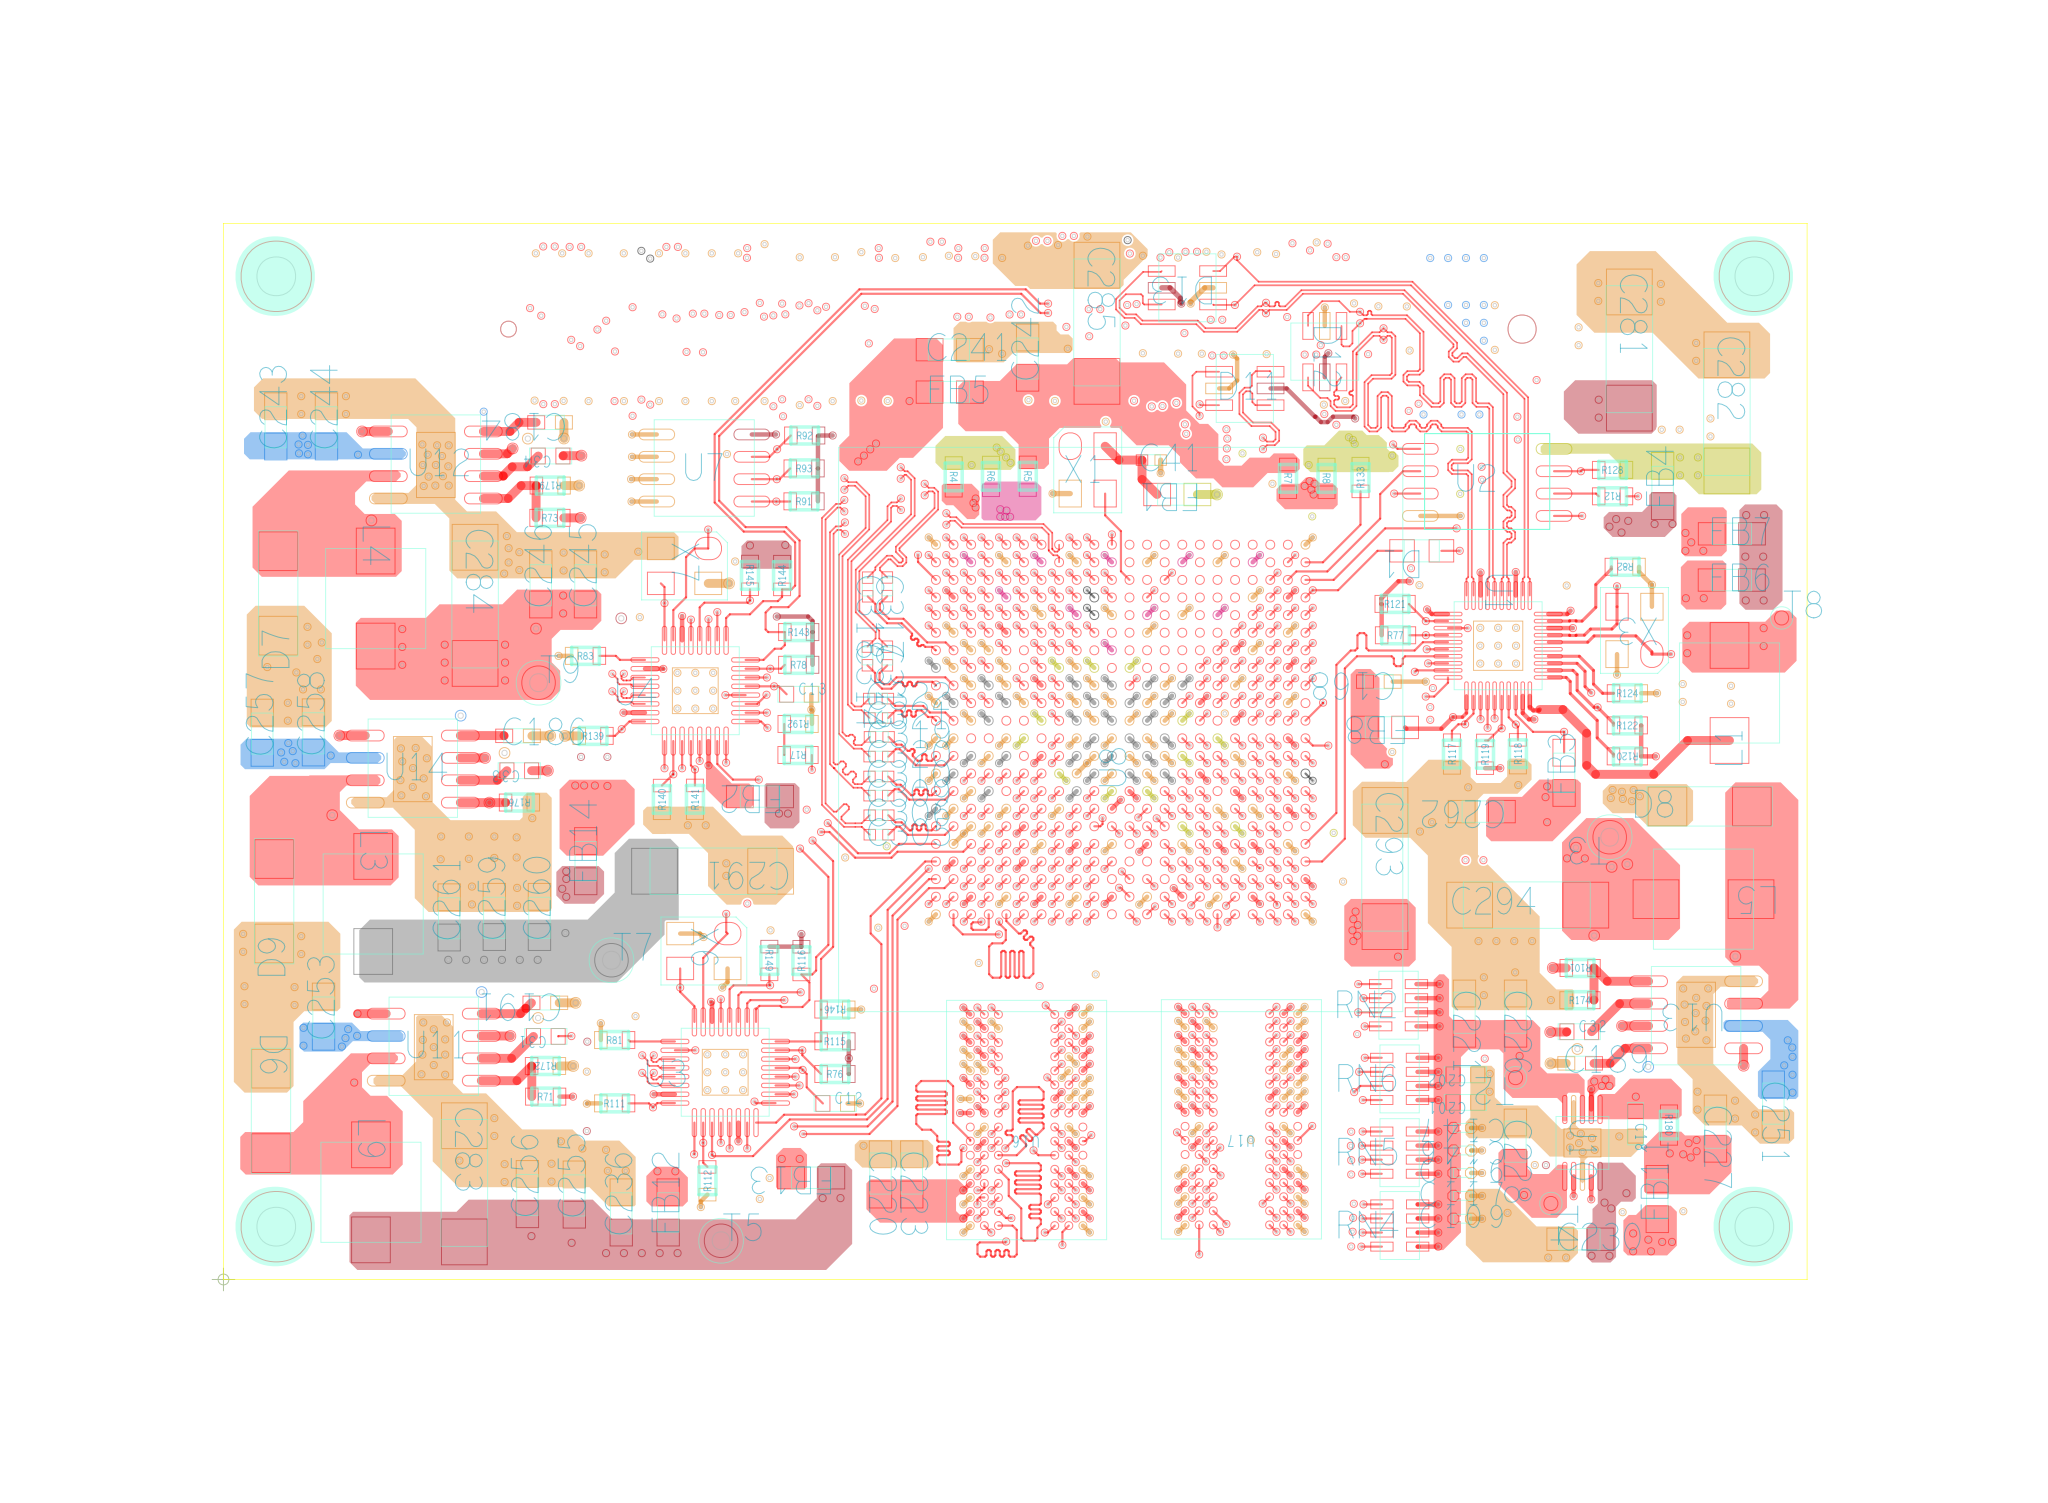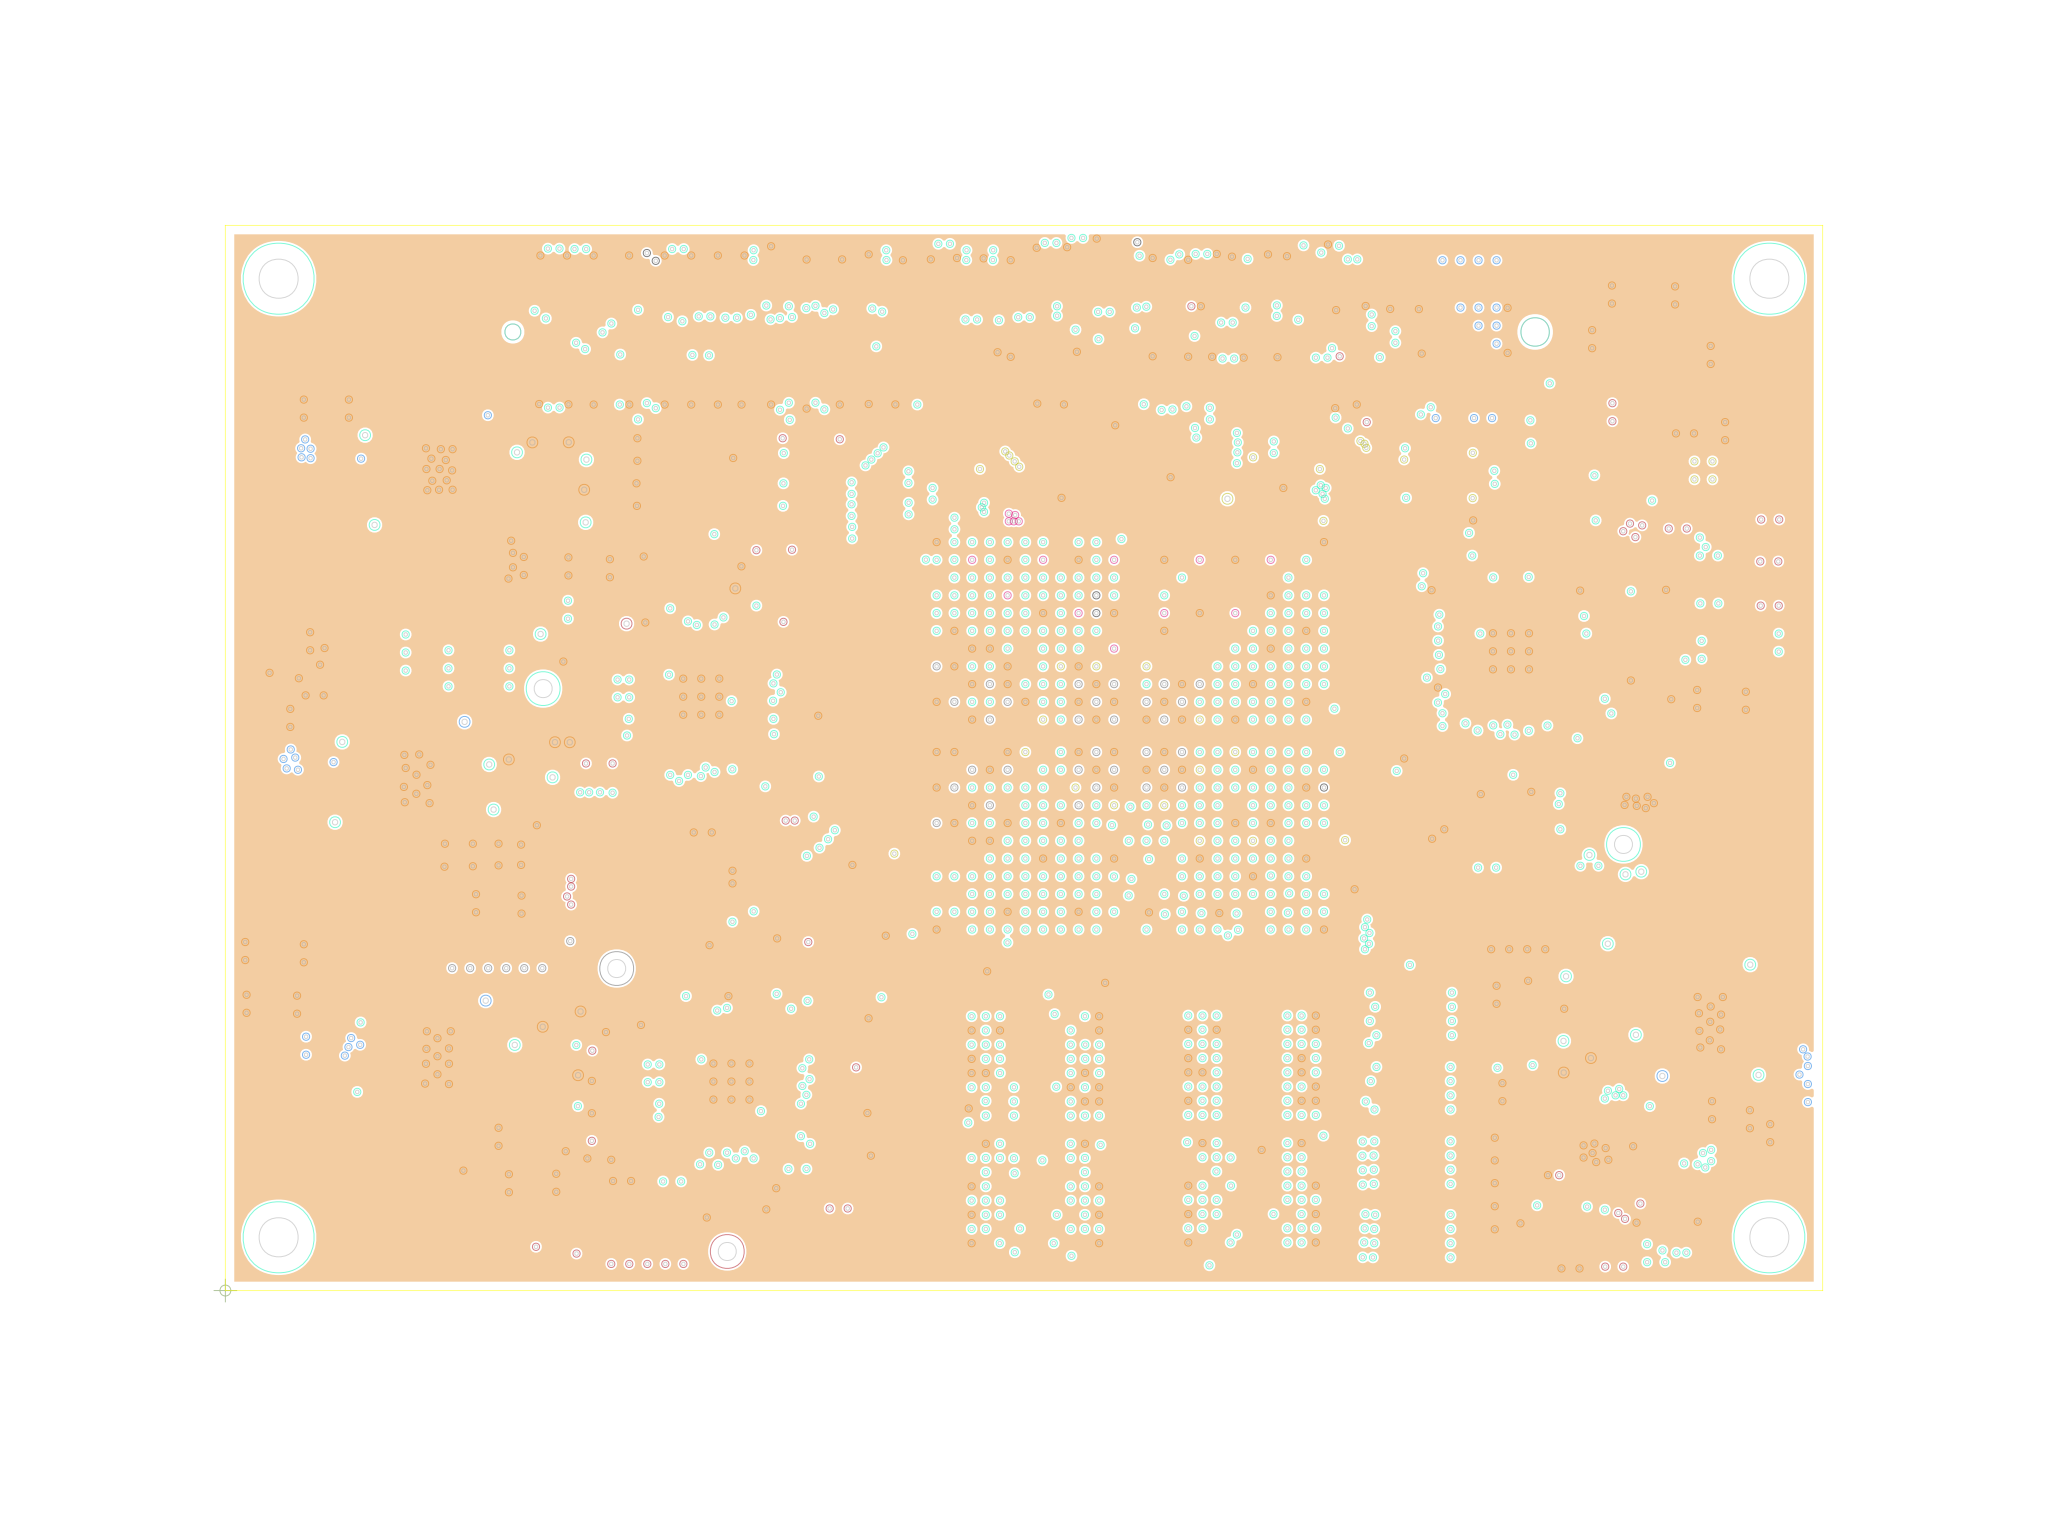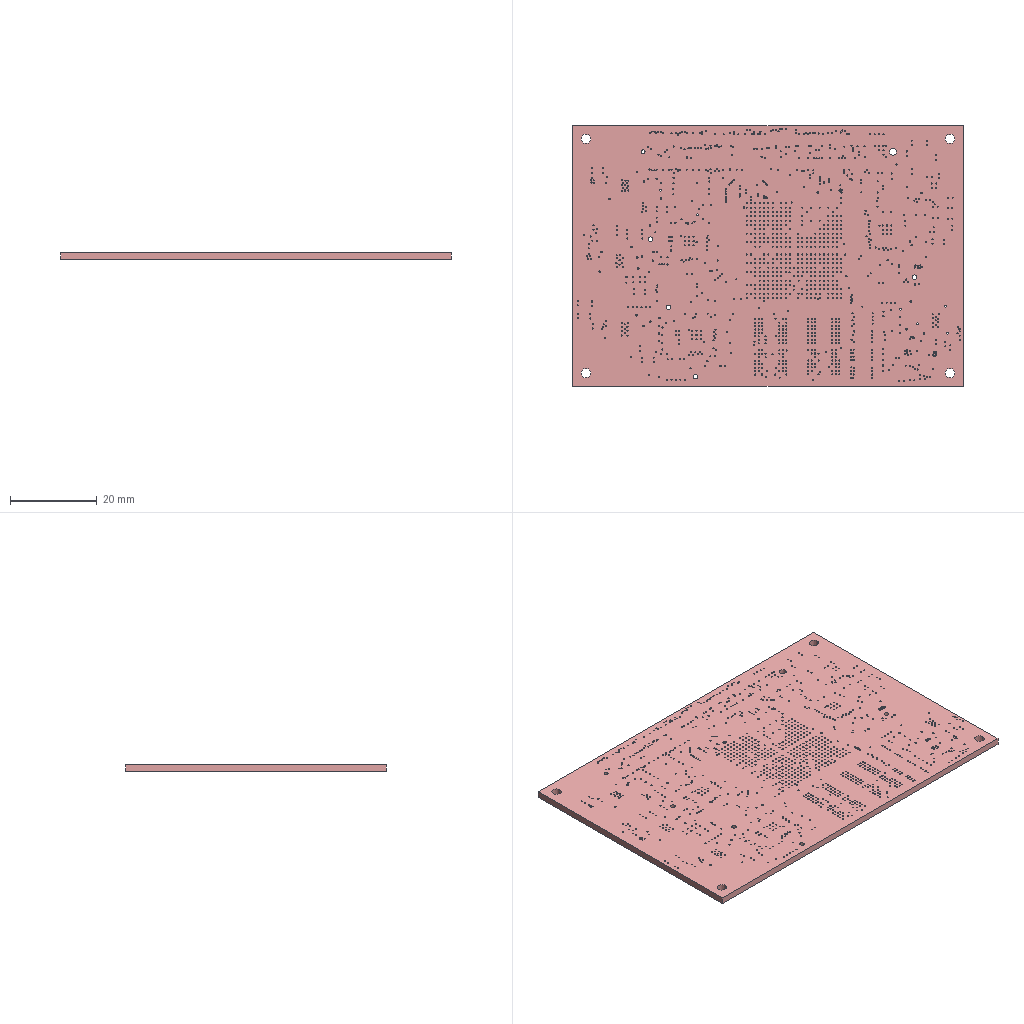Circuit board layout | Cadence Allegro | box 90 x 60 x 1.6 mm
Layer stack:
# Cadence Allegro layer stack of  (unit mm; from the constraint file cross-section; dielectric type: 0 not recorded (Allegro does not mark core vs prepreg), 3 surface material)
index,name,kind,layer,copper_thickness_mm,dielectric_type,dielectric_thickness_mm,dielectric_material,dielectric_constant
0,Top Surface,other,,,,,,
1,TOP,copper,TOP,0.0305,,,,
2,Dielectric1,dielectric,,,0,0.2032,FR-4,4.5
3,GND2,copper,GND2,0.0305,,,,
4,Dielectric2,dielectric,,,0,0.2032,FR-4,4.5
5,SIG3,copper,SIG3,0.0305,,,,
6,Dielectric3,dielectric,,,0,0.2032,FR-4,4.5
7,POWER4,copper,POWER4,0.0305,,,,
8,Dielectric4,dielectric,,,0,0.2032,FR-4,4.5
9,GND5,copper,GND5,0.0305,,,,
10,Dielectric5,dielectric,,,0,0.2032,FR-4,4.5
11,SIG6,copper,SIG6,0.0305,,,,
12,Dielectric6,dielectric,,,0,0.2032,FR-4,4.5
13,POWER7,copper,POWER7,0.0305,,,,
14,Dielectric7,dielectric,,,0,0.2032,FR-4,4.5
15,BOTTOM,copper,BOTTOM,0.0305,,,,
16,Bottom Surface,other,,,,,,
# drill layer pairs: low layer,high layer
drill_pair,TOP,BOTTOM
Part placement:
REFDES,COMP_VALUE,SYM_NAME,SYM_X,SYM_Y,SYM_ROTATE,SYM_MIRROR
C1,10pF,C_0603,1081.558,1609.443,90.000,YES
C2,10pF,C_0603,977.518,1588.167,270.000,YES
C3,10pF,C_0603,1124.854,748.020,90.000,YES
C4,10pF,C_0603,1020.815,726.744,270.000,YES
C6,12pF,C_0603,3147.244,1505.118,180.000,YES
C7,12pF,C_0603,3166.142,1399.606,0.000,YES
C11,100pF,C_0603,2624.185,1510.646,0.000,YES
C12,100pF,C_0603,1368.768,393.717,0.000,NO
C13,100pF,C_0603,1287.652,1309.064,0.000,NO
C14,100pF,C_0603,1655.118,735.654,270.000,YES
C15,100pF,C_0603,2470.000,819.000,90.000,YES
C18,1nF,C_0603,3159.421,348.437,270.000,NO
C21,10nF,C_0603,2905.000,123.999,270.000,YES
C22,10nF,C_0603,364.173,468.110,90.000,YES
C23,10nF,C_0603,3382.724,660.488,270.000,YES
C24,10nF,C_0603,304.504,1066.276,90.000,YES
C25,10nF,C_0603,368.898,1747.472,90.000,YES
C31,22nF,C_0603,721.260,543.701,180.000,NO
C32,22nF,C_0603,3033.465,554.331,0.000,NO
C33,22nF,C_0603,661.811,1138.189,180.000,NO
C34,22nF,C_0603,731.890,1842.126,180.000,NO
C41,100nF_0402,C_0402_104,2076.000,1833.000,0.000,NO
C42,100nF_0402,C_0402_104,3230.000,1849.000,90.000,YES
C44,100nF_0402,C_0402_104,1950.000,1231.000,0.000,YES
C45,100nF_0402,C_0402_104,1866.000,1232.000,0.000,YES
C46,100nF_0402,C_0402_104,1756.000,1273.000,180.000,YES
C47,100nF_0402,C_0402_104,1606.000,1424.000,180.000,YES
C48,100nF_0402,C_0402_104,1600.000,1148.000,0.000,YES
C49,100nF_0402,C_0402_104,1597.000,1335.000,0.000,YES
C50,100nF_0402,C_0402_104,1720.000,1075.000,180.000,YES
C51,100nF_0402,C_0402_104,1892.000,1365.000,270.000,YES
C52,100nF_0402,C_0402_104,985.000,1030.000,180.000,YES
C53,100nF_0402,C_0402_104,2031.000,1231.000,0.000,YES
C54,100nF_0402,C_0402_104,1715.000,1231.000,180.000,YES
C55,100nF_0402,C_0402_104,1599.000,1067.000,180.000,YES
C56,100nF_0402,C_0402_104,1676.000,1186.000,180.000,YES
C57,100nF_0402,C_0402_104,2112.000,1231.000,180.000,YES
C58,100nF_0402,C_0402_104,2010.000,1174.000,90.000,YES
C59,100nF_0402,C_0402_104,1715.000,1345.000,180.000,YES
C60,100nF_0402,C_0402_104,2100.000,1305.000,0.000,YES
C61,100nF_0402,C_0402_104,2120.000,1135.000,270.000,YES
C62,100nF_0402,C_0402_104,2080.000,1135.000,90.000,YES
C63,100nF_0402,C_0402_104,1930.000,1135.000,270.000,YES
C64,100nF_0402,C_0402_104,2100.000,1195.000,0.000,YES
C65,100nF_0402,C_0402_104,1935.000,1325.000,270.000,YES
C66,100nF_0402,C_0402_104,1740.000,1170.000,270.000,YES
C67,100nF_0402,C_0402_104,1970.000,1135.000,90.000,YES
C68,100nF_0402,C_0402_104,1890.000,1170.000,270.000,YES
C69,100nF_0402,C_0402_104,2140.000,1345.000,0.000,YES
C70,100nF_0402,C_0402_104,2045.000,1135.000,270.000,YES
C71,100nF_0402,C_0402_104,1950.000,1195.000,180.000,YES
C72,100nF_0402,C_0402_104,1625.000,1230.000,0.000,YES
C73,100nF_0402,C_0402_104,2010.000,1292.000,90.000,YES
C74,100nF_0402,C_0402_104,2062.000,928.000,0.000,YES
C75,100nF_0402,C_0402_104,1580.000,215.000,270.000,YES
C76,100nF_0402,C_0402_104,1951.000,998.000,180.000,YES
C77,100nF_0402,C_0402_104,2400.000,690.000,180.000,YES
C78,100nF_0402,C_0402_104,1580.000,120.000,90.000,YES
C79,100nF_0402,C_0402_104,2055.000,115.000,90.000,YES
C80,100nF_0402,C_0402_104,2500.000,481.000,90.000,YES
C81,100nF_0402,C_0402_104,2283.000,820.000,90.000,YES
C82,100nF_0402,C_0402_104,2495.000,105.000,90.000,YES
C83,100nF_0402,C_0402_104,2500.000,565.000,270.000,YES
C84,100nF_0402,C_0402_104,2260.000,1265.000,0.000,YES
C85,100nF_0402,C_0402_104,2300.000,1425.000,180.000,YES
C86,100nF_0402,C_0402_104,2465.000,1685.000,90.000,YES
C87,100nF_0402,C_0402_104,2460.000,890.000,180.000,YES
C88,100nF_0402,C_0402_104,2400.000,1565.000,270.000,YES
C89,100nF_0402,C_0402_104,2510.000,1430.000,270.000,YES
C90,100nF_0402,C_0402_104,2240.000,1060.000,90.000,YES
C91,100nF_0402,C_0402_104,2300.000,940.000,45.000,YES
C92,100nF_0402,C_0402_104,2470.000,1430.000,270.000,YES
C93,100nF_0402,C_0402_104,2465.000,1585.000,270.000,YES
C94,100nF_0402,C_0402_104,2395.000,980.000,90.000,YES
C95,100nF_0402,C_0402_104,2035.000,1622.000,180.000,YES
C96,100nF_0402,C_0402_104,2013.000,1527.000,90.000,YES
C97,100nF_0402,C_0402_104,2203.000,1592.000,180.000,YES
C98,100nF_0402,C_0402_104,2035.000,1655.000,180.000,YES
C99,100nF_0402,C_0402_104,2035.000,1589.000,180.000,YES
C100,100nF_0402,C_0402_104,2214.000,1473.000,0.000,YES
C101,100nF_0402,C_0402_104,1992.000,1464.000,180.000,YES
C102,100nF_0402,C_0402_104,2212.000,1529.000,0.000,YES
C103,100nF_0402,C_0402_104,2131.000,1529.000,180.000,YES
C104,100nF_0402,C_0402_104,2202.000,1649.000,180.000,YES
C105,100nF_0402,C_0402_104,1800.000,1145.000,0.000,YES
C106,100nF_0402,C_0402_BGA,2771.000,494.000,0.000,YES
C107,100nF_0402,C_0402_BGA,2770.933,394.571,180.000,YES
C108,100nF_0402,C_0402_BGA,2770.866,83.071,180.000,YES
C109,100nF_0402,C_0402_BGA,2771.654,135.827,0.000,NO
C110,100nF_0402,C_0402_BGA,2771.260,135.433,180.000,YES
C111,100nF_0402,C_0402_BGA,2771.654,187.402,180.000,YES
C112,100nF_0402,C_0402_BGA,2771.260,238.189,180.000,YES
C113,100nF_0402,C_0402_BGA,2771.654,288.583,180.000,YES
C114,100nF_0402,C_0402_BGA,2770.866,338.976,180.000,YES
C115,100nF_0402,C_0402_BGA,2770.866,443.701,180.000,YES
C116,100nF_0402,C_0402_BGA,2771.654,238.189,0.000,NO
C117,100nF_0402,C_0402_BGA,2771.654,187.008,0.000,NO
C121,100nF_0402,C_0402_BGA,1822.033,216.529,270.000,YES
C122,100nF_0402,C_0402_BGA,2685.000,760.000,270.000,YES
C123,100nF_0402,C_0402_BGA,1622.001,216.000,90.000,YES
C124,100nF_0402,C_0402_BGA,1973.001,585.000,90.000,YES
C125,100nF_0402,C_0402_BGA,1973.001,496.000,90.000,YES
C126,100nF_0402,C_0402_BGA,1973.001,408.000,90.000,YES
C127,100nF_0402,C_0402_BGA,2096.000,526.000,270.000,YES
C128,100nF_0402,C_0402_BGA,2096.000,615.000,270.000,YES
C129,100nF_0402,C_0402_BGA,2100.000,215.000,90.000,YES
C130,100nF_0402,C_0402_BGA,2099.000,116.000,270.000,YES
C131,100nF_0402,C_0402_BGA,1618.000,480.000,90.000,YES
C132,100nF_0402,C_0402_BGA,2022.000,586.000,90.000,YES
C133,100nF_0402,C_0402_BGA,1834.000,404.000,90.000,YES
C134,100nF_0402,C_0402_BGA,1618.000,568.000,90.000,YES
C135,100nF_0402,C_0402_BGA,2456.000,474.000,270.000,YES
C136,100nF_0402,C_0402_BGA,2455.000,565.000,90.000,YES
C137,100nF_0402,C_0402_BGA,2452.000,107.000,270.000,YES
C138,100nF_0402,C_0402_BGA,2400.000,646.000,0.000,YES
C139,100nF_0402,C_0402_BGA,1622.000,119.000,270.000,YES
C140,100nF_0402,C_0402_BGA,1978.000,110.000,270.000,YES
C141,100nF_0402,C_0402_BGA,3241.000,133.000,90.000,YES
C142,100nF_0402,C_0402_BGA,3237.008,337.402,90.000,YES
C143,100nF_0402,C_0402_BGA,2900.000,600.000,90.000,YES
C144,100nF_0402,C_0402_BGA,2910.000,235.000,90.000,YES
C145,100nF_0402,C_0402_BGA,3085.000,120.000,90.000,YES
C146,100nF_0402,C_0402_BGA,2772.047,288.583,180.000,NO
C147,100nF_0402,C_0402_BGA,2771.654,338.976,180.000,NO
C148,100nF_0402,C_0402_BGA,2298.815,266.665,90.000,YES
C149,100nF_0402,C_0402_BGA,1618.164,391.728,90.000,YES
C150,100nF_0402,C_0402_BGA,2094.484,393.169,90.000,YES
C151,100nF_0402,C_0402_104,1807.000,1208.000,270.000,YES
C153,100nF_0402,C_0402_104,1795.000,1325.000,45.000,YES
C154,100nF_0402,C_0402_104,1720.000,1445.000,45.000,YES
C155,100nF_0402,C_0402_104,1559.000,1583.000,0.000,YES
C156,100nF_0402,C_0402_104,1774.000,1405.000,90.000,YES
C161,100nF_0603,C_0603_104,2964.244,1383.173,270.000,YES
C162,100nF_0603,C_0603_104,2964.890,1521.362,90.000,YES
C163,100nF_0603,C_0603_104,2890.622,1516.228,270.000,YES
C164,100nF_0603,C_0603_104,2738.654,1457.362,270.000,YES
C165,100nF_0603,C_0603_104,2811.488,1515.819,270.000,YES
C166,100nF_0603,C_0603_104,3413.850,1360.890,270.000,YES
C167,100nF_0603,C_0603_104,2503.000,1159.000,0.000,YES
C168,100nF_0603,C_0603_104,2585.039,1337.402,180.000,NO
C169,100nF_0603,C_0603_104,2675.000,1150.000,180.000,YES
C170,100nF_0603,C_0603_104,2898.102,1171.488,270.000,YES
C171,100nF_0603,C_0603_104,2999.677,1146.480,270.000,YES
C172,100nF_0603,C_0603_104,1038.000,387.000,180.000,YES
C173,100nF_0603,C_0603_104,1029.520,589.047,0.000,YES
C174,100nF_0603,C_0603_104,1011.346,481.299,90.000,YES
C175,100nF_0603,C_0603_104,1074.000,695.000,270.000,YES
C176,100nF_0603,C_0603_104,1170.000,215.000,270.000,YES
C177,100nF_0603,C_0603_104,942.835,1193.488,90.000,YES
C178,100nF_0603,C_0603_104,1053.536,1205.118,180.000,YES
C179,100nF_0603,C_0603_104,962.583,1442.591,0.000,YES
C180,100nF_0603,C_0603_104,944.410,1334.843,90.000,YES
C181,100nF_0603,C_0603_104,1107.071,1442.055,180.000,YES
C182,100nF_0603,C_0603_104,1177.925,1860.079,90.000,YES
C183,100nF_0603,C_0603_104,233.173,1922.165,270.000,YES
C184,100nF_0603,C_0603_104,730.709,1917.323,180.000,NO
C185,100nF_0603,C_0603_104,204.094,1237.638,270.000,YES
C186,100nF_0603,C_0603_104,659.055,1216.142,0.000,NO
C187,100nF_0603,C_0603_104,606.000,815.000,270.000,YES
C188,100nF_0603,C_0603_104,3468.000,557.000,270.000,YES
C189,100nF_0603,C_0603_104,3035.433,483.465,0.000,NO
C190,100nF_0603,C_0603_104,3035.039,625.984,0.000,YES
C191,100nF_0603,C_0603_104,720.079,618.898,180.000,NO
C192,100nF_0603,C_0603_104,780.000,150.000,90.000,YES
C193,100nF_0603,C_0603_104,226.646,601.772,270.000,YES
C201,1uF,C_0603,2778.740,396.063,180.000,NO
C202,1uF,C_0603,2778.740,457.874,180.000,NO
C203,1uF,C_0603,1784.999,400.000,90.000,YES
C204,1uF,C_0603,1530.000,110.000,270.000,YES
C205,1uF,C_0603,1530.000,225.000,90.000,YES
C206,1uF,C_0603,2050.000,220.001,90.000,YES
C207,1uF,C_0603,2033.090,399.736,90.000,YES
C208,1uF,C_0603,1556.377,399.696,90.000,YES
C220,10uF/25V,C_0805_106,1470.000,235.000,270.000,NO
C221,10uF/25V,C_0805_106,2776.563,594.669,270.000,NO
C222,10uF/25V,C_0805_106,2776.000,625.000,90.000,YES
C223,10uF/25V,C_0805_106,1540.000,235.000,270.000,NO
C224,10uF/25V,C_0805_106,1440.000,205.000,90.000,YES
C225,10uF/25V,C_0805_106,2540.000,710.000,180.000,YES
C226,10uF/25V,C_0805_106,2890.925,594.732,270.000,NO
C227,10uF/25V,C_0805_106,3338.169,337.457,270.000,NO
C228,10uF/25V,C_0805_106,2890.531,306.165,270.000,NO
C229,10uF/25V,C_0805_106,3338.583,337.402,90.000,YES
C230,10uF/25V,C_0805_106,3036.000,90.000,0.000,NO
C231,10uF/25V,C_0805_106,3375.079,1564.559,0.000,YES
C232,10uF/25V,C_0805_106,3373.614,1668.760,0.000,YES
C233,10uF/25V,C_0805_106,3313.406,1357.961,90.000,YES
C234,10uF/25V,C_0805_106,2598.819,1235.039,180.000,YES
C236,10uF/25V,C_0805_106,890.000,150.000,90.000,NO
C237,10uF/25V,C_0805_106,1255.000,150.000,270.000,YES
C238,10uF/25V,C_0805_106,809.823,935.331,270.000,YES
C239,10uF/25V,C_0805_106,1199.913,1081.083,0.000,YES
C240,10uF/25V,C_0805_106,3365.748,1853.543,270.000,YES
C241,10uF/25V,C_0805_106,1625.000,2080.000,0.000,NO
C242,10uF/25V,C_0805_106,1799.213,2062.205,90.000,NO
C243,10uF/25V,C_0805_106,117.031,1908.386,90.000,NO
C244,10uF/25V,C_0805_106,230.417,1908.386,90.000,NO
C245,10uF/25V,C_0805_106,810.000,1555.000,90.000,NO
C246,10uF/25V,C_0805_106,710.000,1555.000,90.000,NO
C247,10uF/25V,C_0805_106,3011.024,851.575,90.000,YES
C248,10uF/25V,C_0805_106,2799.213,847.638,90.000,YES
C249,10uF/25V,C_0805_106,2907.480,846.457,90.000,YES
C250,10uF/25V,C_0805_106,3468.394,390.976,90.000,YES
C251,10uF/25V,C_0805_106,3467.606,391.370,270.000,NO
C252,10uF/25V,C_0805_106,99.087,587.205,270.000,YES
C253,10uF/25V,C_0805_106,223.890,587.992,90.000,NO
C254,10uF/25V,C_0805_106,871.000,152.000,270.000,YES
C255,10uF/25V,C_0805_106,785.000,190.000,90.000,NO
C256,10uF/25V,C_0805_106,680.000,191.000,90.000,NO
C257,10uF/25V,C_0805_106,86.772,1223.071,90.000,NO
C258,10uF/25V,C_0805_106,201.339,1223.858,90.000,NO
C259,10uF/25V,C_0805_106,606.000,811.000,90.000,NO
C260,10uF/25V,C_0805_106,707.000,811.000,90.000,NO
C261,10uF/25V,C_0805_106,505.000,810.000,90.000,NO
C262,10uF/25V,C_0805_106,2815.378,1046.626,180.000,NO
C281,100uF/6.3Vdc,C_7343,3145.563,2079.149,270.000,NO
C282,100uF/6.3Vdc,C_7343,3363.780,1938.583,270.000,NO
C283,100uF/6.3Vdc,C_7343,539.000,213.999,270.000,NO
C284,100uF/6.3Vdc,C_7343,563.000,1507.999,270.000,NO
C285,100uF/6.3Vdc,C_7343,1954.331,2138.976,270.000,NO
C291,330uF/2.5Vdc,C_7343,1094.338,913.202,180.000,NO
C292,330uF/2.5Vdc,C_7343,1092.901,912.989,0.000,YES
C293,330uF/2.5Vdc,C_7343,2598.819,919.290,270.000,NO
C294,330uF/2.5Vdc,C_7343,2918.110,837.402,0.000,NO
C302,10uF/25V,C_0805_106,3143.595,1994.897,270.000,YES
C303,100nF_0402,C_0402_104,1466.550,1081.918,180.000,YES
C304,100nF_0402,C_0402_104,1466.550,1125.225,180.000,YES
C305,100nF_0402,C_0402_104,1466.944,994.910,0.000,NO
C306,100nF_0402,C_0402_104,1466.629,1038.595,0.000,NO
C307,100nF_0402,C_0402_104,1466.550,1169.713,180.000,YES
C308,100nF_0402,C_0402_104,1467.337,1213.808,180.000,YES
C309,100nF_0402,C_0402_104,1466.456,1082.296,0.000,NO
C310,100nF_0402,C_0402_104,1466.267,1125.209,0.000,NO
C311,100nF_0402,C_0402_104,1465.369,1344.910,180.000,YES
C312,100nF_0402,C_0402_104,1466.156,1389.792,180.000,YES
C313,100nF_0402,C_0402_104,1485.298,1394.693,270.000,NO
C314,100nF_0402,C_0402_104,1440.809,1394.882,270.000,NO
C315,100nF_0402,C_0402_104,1466.156,1435.067,180.000,YES
C316,100nF_0402,C_0402_104,1465.369,1479.162,180.000,YES
C317,100nF_0402,C_0402_104,1485.230,1549.503,270.000,NO
C318,100nF_0402,C_0402_104,1441.371,1549.125,270.000,NO
C319,100nF_0402,C_0402_104,1467.338,1213.841,0.000,NO
C320,100nF_0402,C_0402_104,1466.549,1169.680,0.000,NO
C321,100nF_0402,C_0402_104,1466.204,1256.091,0.000,NO
C322,100nF_0402,C_0402_104,1465.621,1299.398,0.000,NO
D1,R_LED_SMT,D_LED0805,2681.001,1630.001,180.000,NO
D6,SS210,DO214,106.299,377.165,270.000,NO
D7,SS210,DO214,122.441,1534.646,90.000,NO
D8,SS210,DO214,3325.197,1058.268,0.000,NO
D9,SS210,DO214,113.386,846.063,90.000,NO
D11,SRV05-4,D_SOT23_6,2285.200,1993.246,0.000,NO
D12,SRV05-4,D_SOT23_6,2464.076,2075.592,270.000,NO
D13,SRV05-4,D_SOT23_6,2156.756,2218.426,180.000,NO
FB1,CBW201209U600T,L_0805,2134.000,1756.000,180.000,NO
FB2,CBW201209U600T,L_0805,1200.394,1080.315,180.000,NO
FB3,CBW201209U600T,L_0805,2999.524,1133.394,90.000,NO
FB4,CBW201209U600T,L_0805,3220.000,1775.000,90.000,NO
FB5,CBW201209U600T,L_0805,1625.000,1985.000,0.000,NO
FB6,CBW201209U600T,L_0805,3374.685,1564.559,0.000,NO
FB7,CBW201209U600T,L_0805,3374.898,1668.055,0.000,NO
FB8,CBW201209U600T,L_0805,2598.732,1234.957,180.000,NO
FB10,CBW201209U600T,L_0805,2604.331,874.409,90.000,YES
FB11,CBW201209U600T,L_0805,3208.000,180.000,90.000,NO
FB12,CBW201209U600T,L_0805,995.000,150.000,90.000,NO
FB13,CBW201209U600T,L_0805,1314.961,227.559,180.000,NO
FB14,CBW201209U600T,L_0805,810.547,935.787,90.000,NO
J10,COM_E connector 220X8 FEMALE,JP_220X8PF,1771.654,2125.984,90.000,YES
L1,2.2uH,L_SDB0530,3369.642,1312.016,90.000,NO
L3,3.3uH,L_SDB0530,335.000,840.000,270.000,NO
L4,3.3uH,L_SDB0530,340.551,1523.228,270.000,NO
L5,3.3uH,L_SDB0530,3311.417,850.787,180.000,NO
L9,4.7uH,L_SDB0530,330.000,195.000,270.000,NO
R1,0,R_0603,1582.677,732.110,90.000,YES
R2,0,R_0603,2184.506,710.691,90.000,YES
R3,0,R_0603,1782.286,713.774,270.000,YES
R4,0,R_0603,1633.858,1795.410,270.000,NO
R5,0,R_0603,1799.606,1796.850,270.000,NO
R6,0,R_0603,1717.154,1796.457,270.000,NO
R7,0,R_0603,2381.890,1792.126,270.000,NO
R8,0,R_0603,2468.000,1792.000,270.000,NO
R9,0,R_0603,2105.000,1400.000,0.000,YES
R10,0,R_0603,2009.000,1383.000,90.000,YES
R11,10,R_0603,3015.000,129.000,270.000,YES
R12,10,R_0603,3108.000,1752.000,180.000,NO
R13,10,R_0603,364.173,587.402,270.000,YES
R14,10,R_0603,3382.724,541.197,90.000,YES
R15,10,R_0603,304.504,1185.567,270.000,YES
R16,10,R_0603,368.898,1866.764,270.000,YES
R17,10,R_0603,1285.505,1173.281,180.000,NO
R21,33.2,R_0603,2632.323,407.066,0.000,YES
R22,33.2,R_0603,2632.039,478.325,0.000,YES
R23,33.2,R_0603,2630.873,548.778,180.000,YES
R26,499,R_0603,659.843,1138.189,180.000,YES
R31,80.6,R_0603,878.000,532.000,0.000,YES
R32,80.6,R_0603,877.000,332.000,0.000,YES
R41,49.9,R_0603,854.000,1448.000,270.000,YES
R42,49.9,R_0603,794.000,1448.000,270.000,YES
R43,49.9,R_0603,859.000,1228.000,90.000,YES
R44,49.9,R_0603,800.000,1228.000,90.000,YES
R51,130,R_0603,876.717,393.248,180.000,YES
R52,130,R_0603,877.220,464.902,180.000,YES
R56,243,R_0603,1986.271,228.346,90.000,YES
R57,243,R_0603,2466.528,233.464,90.000,YES
R58,243,R_0603,1852.217,713.790,270.000,YES
R59,243,R_0603,1921.222,713.397,270.000,YES
R61,1K,R_0603,2955.000,129.000,90.000,YES
R62,1K,R_0603,2688.000,1628.000,180.000,YES
R64,1K,R_0603,2397.000,1715.000,270.000,YES
R65,1K,R_0603,2338.000,1715.000,270.000,YES
R66,1K,R_0603,1425.000,913.000,270.000,YES
R67,1K,R_0603,1484.000,913.000,90.000,YES
R71,1.21K,R_0603,720.866,409.055,0.000,NO
R73,1.24K,R_0603,730.449,1703.736,0.000,NO
R76,1.5K,R_0603,1368.134,459.642,0.000,NO
R77,1.5K,R_0603,2622.354,1441.138,0.000,NO
R78,1.5K,R_0603,1287.019,1374.989,0.000,NO
R81,2.49K,R_0603,875.283,535.626,0.000,NO
R82,2.49K,R_0603,3136.244,1594.295,180.000,NO
R83,2.49K,R_0603,810.000,1395.000,0.000,NO
R91,3.32K,R_0603,1298.969,1740.744,0.000,NO
R92,3.32K,R_0603,1300.433,1887.988,0.000,NO
R93,3.32K,R_0603,1299.142,1814.366,0.000,NO
R94,3.32K,R_0603,3036.220,553.543,0.000,YES
R95,3.32K,R_0603,729.134,1842.913,180.000,YES
R96,3.32K,R_0603,718.504,544.488,180.000,YES
R101,4.02K,R_0603,3035.433,696.850,180.000,NO
R111,4.75K,R_0603,875.300,394.000,0.000,NO
R112,4.75K,R_0603,1082.846,220.748,90.000,NO
R113,4.75K,R_0603,1103.000,210.000,270.000,YES
R115,4.75K,R_0603,1368.165,532.902,0.000,NO
R116,4.75K,R_0603,1293.083,713.331,90.000,NO
R117,4.75K,R_0603,2748.594,1175.425,90.000,NO
R118,4.75K,R_0603,2896.232,1176.102,90.000,NO
R119,4.75K,R_0603,2822.610,1174.811,90.000,NO
R120,4.75K,R_0603,3140.968,1170.180,180.000,NO
R121,4.75K,R_0603,2621.441,1511.248,0.000,NO
R122,4.75K,R_0603,3140.952,1239.506,0.000,NO
R123,4.75K,R_0603,3140.944,1239.424,180.000,YES
R124,4.75K,R_0603,3141.126,1311.500,0.000,NO
R125,4.75K,R_0603,1524.000,732.000,270.000,YES
R126,4.75K,R_0603,2687.555,1857.868,180.000,YES
R127,4.75K,R_0603,2687.161,1757.473,180.000,YES
R128,4.75K,R_0603,3108.000,1811.000,0.000,NO
R132,4.75K,R_0603,2521.000,969.000,270.000,YES
R133,4.75K,R_0603,2544.000,1794.000,90.000,NO
R134,4.75K,R_0603,2448.000,968.000,270.000,YES
R139,4.75K,R_0603,827.000,1216.000,0.000,NO
R140,4.75K,R_0603,980.878,1073.898,90.000,NO
R141,4.75K,R_0603,1054.894,1074.181,90.000,NO
R142,4.75K,R_0603,1177.881,1575.211,90.000,YES
R143,4.75K,R_0603,1287.050,1448.249,0.000,NO
R144,4.75K,R_0603,1249.786,1574.754,90.000,NO
R145,4.75K,R_0603,1178.046,1575.037,270.000,NO
R146,4.75K,R_0603,1368.008,603.854,180.000,NO
R147,4.75K,R_0603,1224.000,720.000,90.000,YES
R148,4.75K,R_0603,3035.827,696.850,180.000,YES
R149,4.75K,R_0603,1221.343,713.614,270.000,NO
R161,5.11K,R_0603,662.205,1066.929,180.000,YES
R171,10K,R_0603,577.559,575.591,90.000,YES
R172,10K,R_0603,720.472,477.559,180.000,NO
R173,10K,R_0603,3187.795,536.220,270.000,YES
R174,10K,R_0603,3035.039,624.803,0.000,NO
R175,10K,R_0603,530.709,1197.638,90.000,YES
R176,10K,R_0603,662.205,1066.929,180.000,NO
R177,10K,R_0603,2989.890,221.768,180.000,YES
R178,10K,R_0603,582.283,1877.953,90.000,YES
R179,10K,R_0603,731.102,1775.984,180.000,NO
R180,10K,R_0603,3234.193,345.425,270.000,NO
R181,10K,R_0603,3228.000,419.000,180.000,YES
R191,20K,R_0603,730.291,1703.878,0.000,YES
R192,20K,R_0603,1285.710,1242.683,180.000,NO
R196,30.1K,R_0603,720.079,409.055,0.000,YES
R199,100K,R_0603,3108.000,221.000,180.000,YES
R200,4.75K,R_0603,3140.968,1311.626,180.000,YES
R201,4.75K,R_0603,1465.000,732.000,90.000,YES
RN1,33,RESNET4,2631.511,283.734,180.000,YES
RN2,33,RESNET4,2629.147,613.530,0.000,NO
RN3,33,RESNET4,2631.511,121.135,180.000,YES
RN4,33,RESNET4,2631.904,120.742,0.000,NO
RN5,33,RESNET4,2631.511,283.734,0.000,NO
RN6,33,RESNET4,2631.511,448.694,0.000,NO
T1,TP_0_8,TP_0_8,1712.000,732.000,0.000,YES
T2,TP_0_8,TP_0_8,2890.945,451.575,180.000,NO
T3,1.5V 3A,TP,3101.575,989.370,180.000,NO
T4,TP_0_8,TP_0_8,2970.000,170.000,270.000,NO
T5,3.3V  2A,TP,1113.386,86.614,0.000,NO
T7,1.2V 1A,TP,868.110,714.173,0.000,NO
T8,TP_0_8,TP_0_8,3486.220,1479.921,0.000,NO
T9,2.5V 1A,TP,705.000,1335.000,0.000,NO
U1,RTL8211FI-CG,U_QFN40_0_4,2851.969,1417.717,270.000,NO
U2,W25Q64FVSSIG,U_SO8W,2827.436,1783.064,0.000,NO
U3,RTL8201FI-VC-CG,U_QFN32_0_5,1122.606,463.547,0.000,NO
U4,RTL8201FI-VC-CG,U_QFN32_0_5,1055.670,1317.091,0.000,NO
U7,AT24C32D,U_SO8,1075.748,1815.276,0.000,NO
U8,PGL50H-7IFBGA484,U_FBGA484_1_0,2007.480,1230.315,90.000,NO
U10,TPS51200DRCT,U_VSON10,3040.551,305.512,270.000,NO
U11,SGM6130,U_SO8DDA,470.472,519.685,0.000,NO
U12,SGM6130,U_SO8DDA,475.197,1822.047,0.000,NO
U13,SGM6130,U_SO8DDA,3294.882,592.126,180.000,NO
U14,SGM6130,U_SO8DDA,423.622,1141.732,0.000,NO
U16,HXI15H4G160AF-13K,U_TFBGA96,1796.901,356.692,180.000,NO
U17,HXI15H4G160AF-13K,U_TFBGA96,2277.551,358.268,180.000,NO
X1,25MHz,XTAL3225,1933.638,1811.087,0.000,NO
X3,25MHz,XTAL3225,3156.992,1451.906,180.000,NO
X6,25MHz,XTAL3225,1074.866,734.787,270.000,NO
X7,25MHz,XTAL3225,1031.570,1596.211,270.000,NO
Pad and via stacks:
# Allegro (Cadence) via spans and padstacks; design units: ("mils" 3 1000)
# via spans: padstack,start_layer,end_layer,net_example,count
VIA12_24,ETCH/TOP,ETCH/BOTTOM,N20035026,38
VIA-8X16,ETCH/TOP,ETCH/BOTTOM,GND,1368
# Allegro padstack definitions: name,start_layer,end_layer,drill,plating,holeType,type
SMD38_30,"ETCH/TOP","ETCH/TOP",0.0,"PLATED","none","smd"
SMD26_24,"ETCH/TOP","ETCH/TOP",0.0,"PLATED","none","smd"
SMD0R635-OT,"ETCH/TOP","ETCH/TOP",0.0,"PLATED","none","smd"
SMD60_50,"ETCH/TOP","ETCH/TOP",0.0,"PLATED","none","smd"
SMD102_102,"ETCH/TOP","ETCH/TOP",0.0,"PLATED","none","smd"
SMD55_50,"ETCH/TOP","ETCH/TOP",0.0,"PLATED","none","smd"
SMD60_24,"ETCH/TOP","ETCH/TOP",0.0,"NON_PLATED","none","smd"
SMD87_87,"ETCH/TOP","ETCH/TOP",0.0,"PLATED","none","smd"
SMD75_10,"ETCH/TOP","ETCH/TOP",0.0,"PLATED","none","smd"
SMD150_79,"ETCH/TOP","ETCH/TOP",0.0,"PLATED","none","smd"
SMD102_87,"ETCH/TOP","ETCH/TOP",0.0,"NON_PLATED","none","smd"
SMD50_20,"ETCH/TOP","ETCH/TOP",0.0,"NON_PLATED","none","smd"
BALL31,"ETCH/TOP","ETCH/TOP",0.0,"PLATED","none","smd"
SMD63_8OB,"ETCH/TOP","ETCH/TOP",0.0,"NON_PLATED","none","smd"
SMD8_63OB,"ETCH/TOP","ETCH/TOP",0.0,"NON_PLATED","none","smd"
SMD110_110,"ETCH/TOP","ETCH/TOP",0.0,"NON_PLATED","none","smd"
SMD63_10OB,"ETCH/TOP","ETCH/TOP",0.0,"PLATED","none","smd"
SMD63_83,"ETCH/TOP","ETCH/TOP",0.0,"PLATED","none","smd"
SMD85_24OB,"ETCH/TOP","ETCH/TOP",0.0,"PLATED","none","smd"
SMD87_146,"ETCH/TOP","ETCH/TOP",0.0,"NON_PLATED","none","smd"
BALL18,"ETCH/TOP","ETCH/TOP",0.0,"PLATED","none","smd"
SMD80_24OB,"ETCH/TOP","ETCH/TOP",0.0,"NON_PLATED","none","smd"
SMD10_63OB,"ETCH/TOP","ETCH/TOP",0.0,"NON_PLATED","none","smd"
SMD50_60OB,"ETCH/TOP","ETCH/TOP",0.0,"PLATED","none","smd"
SMD50_60,"ETCH/TOP","ETCH/TOP",0.0,"PLATED","none","smd"
S_R0R80X0R90,"ETCH/TOP","ETCH/TOP",0.0,"PLATED","none","smd"
RX0_70Y0_96T,"ETCH/TOP","ETCH/TOP",0.0,"PLATED","none","smd"
Y10,"ETCH/TOP","ETCH/TOP",0.0,"NON_PLATED","none","smd"
S_S0R55,"ETCH/TOP","ETCH/TOP",0.0,"PLATED","none","smd"
R127X120,"ETCH/TOP","ETCH/TOP",0.0,"NON_PLATED","none","smd"
BALL20,"ETCH/TOP","ETCH/TOP",0.0,"NON_PLATED","none","smd"
PAD125CIR63D,"ETCH/TOP","ETCH/BOTTOM",63.0,"PLATED","circle_drill","through"
PTH70CIR35,"ETCH/TOP","ETCH/BOTTOM",35.0,"PLATED","circle_drill","through"
NPTH35CIR35,"ETCH/TOP","ETCH/BOTTOM",35.402,"NON_PLATED","circle_drill","through"
NPTH63CIR63,"ETCH/TOP","ETCH/BOTTOM",63.0,"NON_PLATED","circle_drill","through"
PTH75_75OB40,"ETCH/TOP","ETCH/BOTTOM",40.0,"PLATED","circle_drill","through"
Y300,"ETCH/TOP","ETCH/BOTTOM",125.0,"NON_PLATED","circle_drill","through"
Y2_2,"ETCH/TOP","ETCH/BOTTOM",86.614,"NON_PLATED","circle_drill","through"
BALL40_TB-MARK,"ETCH/TOP","ETCH/BOTTOM",0.0,"PLATED","none","through"
VIA-8X16,"ETCH/TOP","ETCH/BOTTOM",8.0,"PLATED","circle_drill","through"
VIA12_24,"ETCH/TOP","ETCH/BOTTOM",12.0,"PLATED","circle_drill","through"
VIA24D12,"ETCH/TOP","ETCH/BOTTOM",12.0,"PLATED","circle_drill","through"
Design rules, without the lines most boards share, first 14 of 90 lines:
# Cadence Allegro design rules of  (from the Constraint Manager export constraints.dcfx, design unit mil; typed fields in mm)
# columns: name | kind | enabled | priority | scope1 | scope2 | descriptor | typed fields (field=value)
# Allegro precedence (priority 1 wins): 1 Region class-to-class, 2 Region class, 3 Region, 4 class-to-class, 5 DiffPair/Bus/NetGroup override, 6 NetClass, 7 constraint set (CSet) default
# per-layer values are written LAYER=value in the descriptor and LAYER:mm in the typed field; a maximum of 0 means no limit set
# --- net classes (and buses / net groups) ---
DIFF100 | NetClass | enabled | 6 | DDR3_CLK, DIFFIO_B2_15, DIFFIO_B2_16, DIFFIO_B2_17, DIFFIO_B2_18, DIFFIO_B2_19, DIFFIO_B2_30, DIFFIO_B2_31, DIFFIO_B2_32, DIFFIO_B2_33, DIFFIO_B2_34, DIFFIO_B2_35, DIFFIO_B2_53, DIFFI_B1_0, DIFFI_B1_1, DIFFI_B1_11, DIFFI_B1_12, DIFFI_B1_13, DIFFI_B1_22, DIFFPAIR0, DIFFPAIR1, DP1, DP2, DP3, DP4, DP5, DP6, DP7, DP8, DP9, DP10, DP11, DP12, DP13, DP14, GLAN_TRD0, GLAN_TRD1, GLAN_TRD3, RD_A, RD_B, TD_B, DIFFPAIR2, DIFFPAIR3, DIFFPAIR4, DIFFPAIR5, DIFFPAIR6, DIFFPAIR7, DIFFPAIR8, DIFFPAIR9, DIFFPAIR10, DIFFPAIR11, GLAN_TRD2 | All | Net Class (PhysicalCSet=DIFF100) (SpacingCSet=DIFF) (members: 52 DiffPair) | physicalcset=DIFF100 spacingcset=DIFF
PWR | NetClass | enabled | 6 | +12V, AVDD_1V0, AVDD_3V3, AVDD33_A, AVDD33_B, DVDD_3V3, DVDD33_A, DVDD33_B, FPGA_1V2, FPGA_2V5, FPGA_3V3, GND, 1V5, 2V5, 3V3, POW_B0, POW_B1, POW_B2, DDR3_1V5, DDR_VREF, VTT | All | Net Class (PhysicalCSet=PWR) (members: 21 Net) | physicalcset=PWR
GMACRXD | NetGroup | enabled | 5 | GMAC1_RXD3, GMAC1_RXD2, GMAC1_RXD1, GMAC1_RXD0, GMAC1_RXCK, GMAC1_RCTL | All | NetGroup (members: 6 Net) |
GMACTXD | NetGroup | enabled | 5 | GMAC1_TXD3, GMAC1_TXD2, GMAC1_TXD1, GMAC1_TXD0, GMAC1_TXCK, GMAC1_TCTL | All | NetGroup (members: 6 Net) overrides: (DIFFP_PHASE_TOL=5 mil) |  diffp_phase_tol=5mil
ADD | NetGroup | enabled | 5 | DDR3_ODT, DDR3_NWE, DDR3_NRAS, DDR3_NCAS, DDR3_CKE, DDR3_BA2, DDR3_BA1, DDR3_BA0, DDR3_A9, DDR3_A8, DDR3_A7, DDR3_A6, DDR3_A5, DDR3_A4, DDR3_A3, DDR3_A2, DDR3_A15, DDR3_A14, DDR3_A13, DDR3_A12, DDR3_A11, DDR3_A10, DDR3_A1, DDR3_A0, DDR3_CLKN, DDR3_CLKP, DDR3_NSCS | All | NetGroup (members: 27 Net) |
DATA3 | NetGroup | enabled | 5 | DDR3_DQ31, DDR3_DQ30, DDR3_DQ29, DDR3_DQ28, DDR3_DQ27, DDR3_DQ26, DDR3_DQ25, DDR3_DQ24, DDR3_DQM3, DDR3_DQSN3, DDR3_DQSP3 | All | NetGroup (members: 11 Net) |
DATA2 | NetGroup | enabled | 5 | DDR3_DQ23, DDR3_DQ22, DDR3_DQ21, DDR3_DQ20, DDR3_DQ19, DDR3_DQ18, DDR3_DQ17, DDR3_DQ16, DDR3_DQM2, DDR3_DQSN2, DDR3_DQSP2 | All | NetGroup (members: 11 Net) |
DATA1 | NetGroup | enabled | 5 | DDR3_DQ9, DDR3_DQ8, DDR3_DQ15, DDR3_DQ14, DDR3_DQ13, DDR3_DQ12, DDR3_DQ11, DDR3_DQ10, DDR3_DQM1, DDR3_DQSN1, DDR3_DQSP1 | All | NetGroup (members: 11 Net) |
DATA0 | NetGroup | enabled | 5 | DDR3_DQ7, DDR3_DQ6, DDR3_DQ5, DDR3_DQ4, DDR3_DQ3, DDR3_DQ2, DDR3_DQ1, DDR3_DQ0, DDR3_DQM0, DDR3_DQSN0, DDR3_DQSP0 | All | NetGroup (members: 11 Net) |